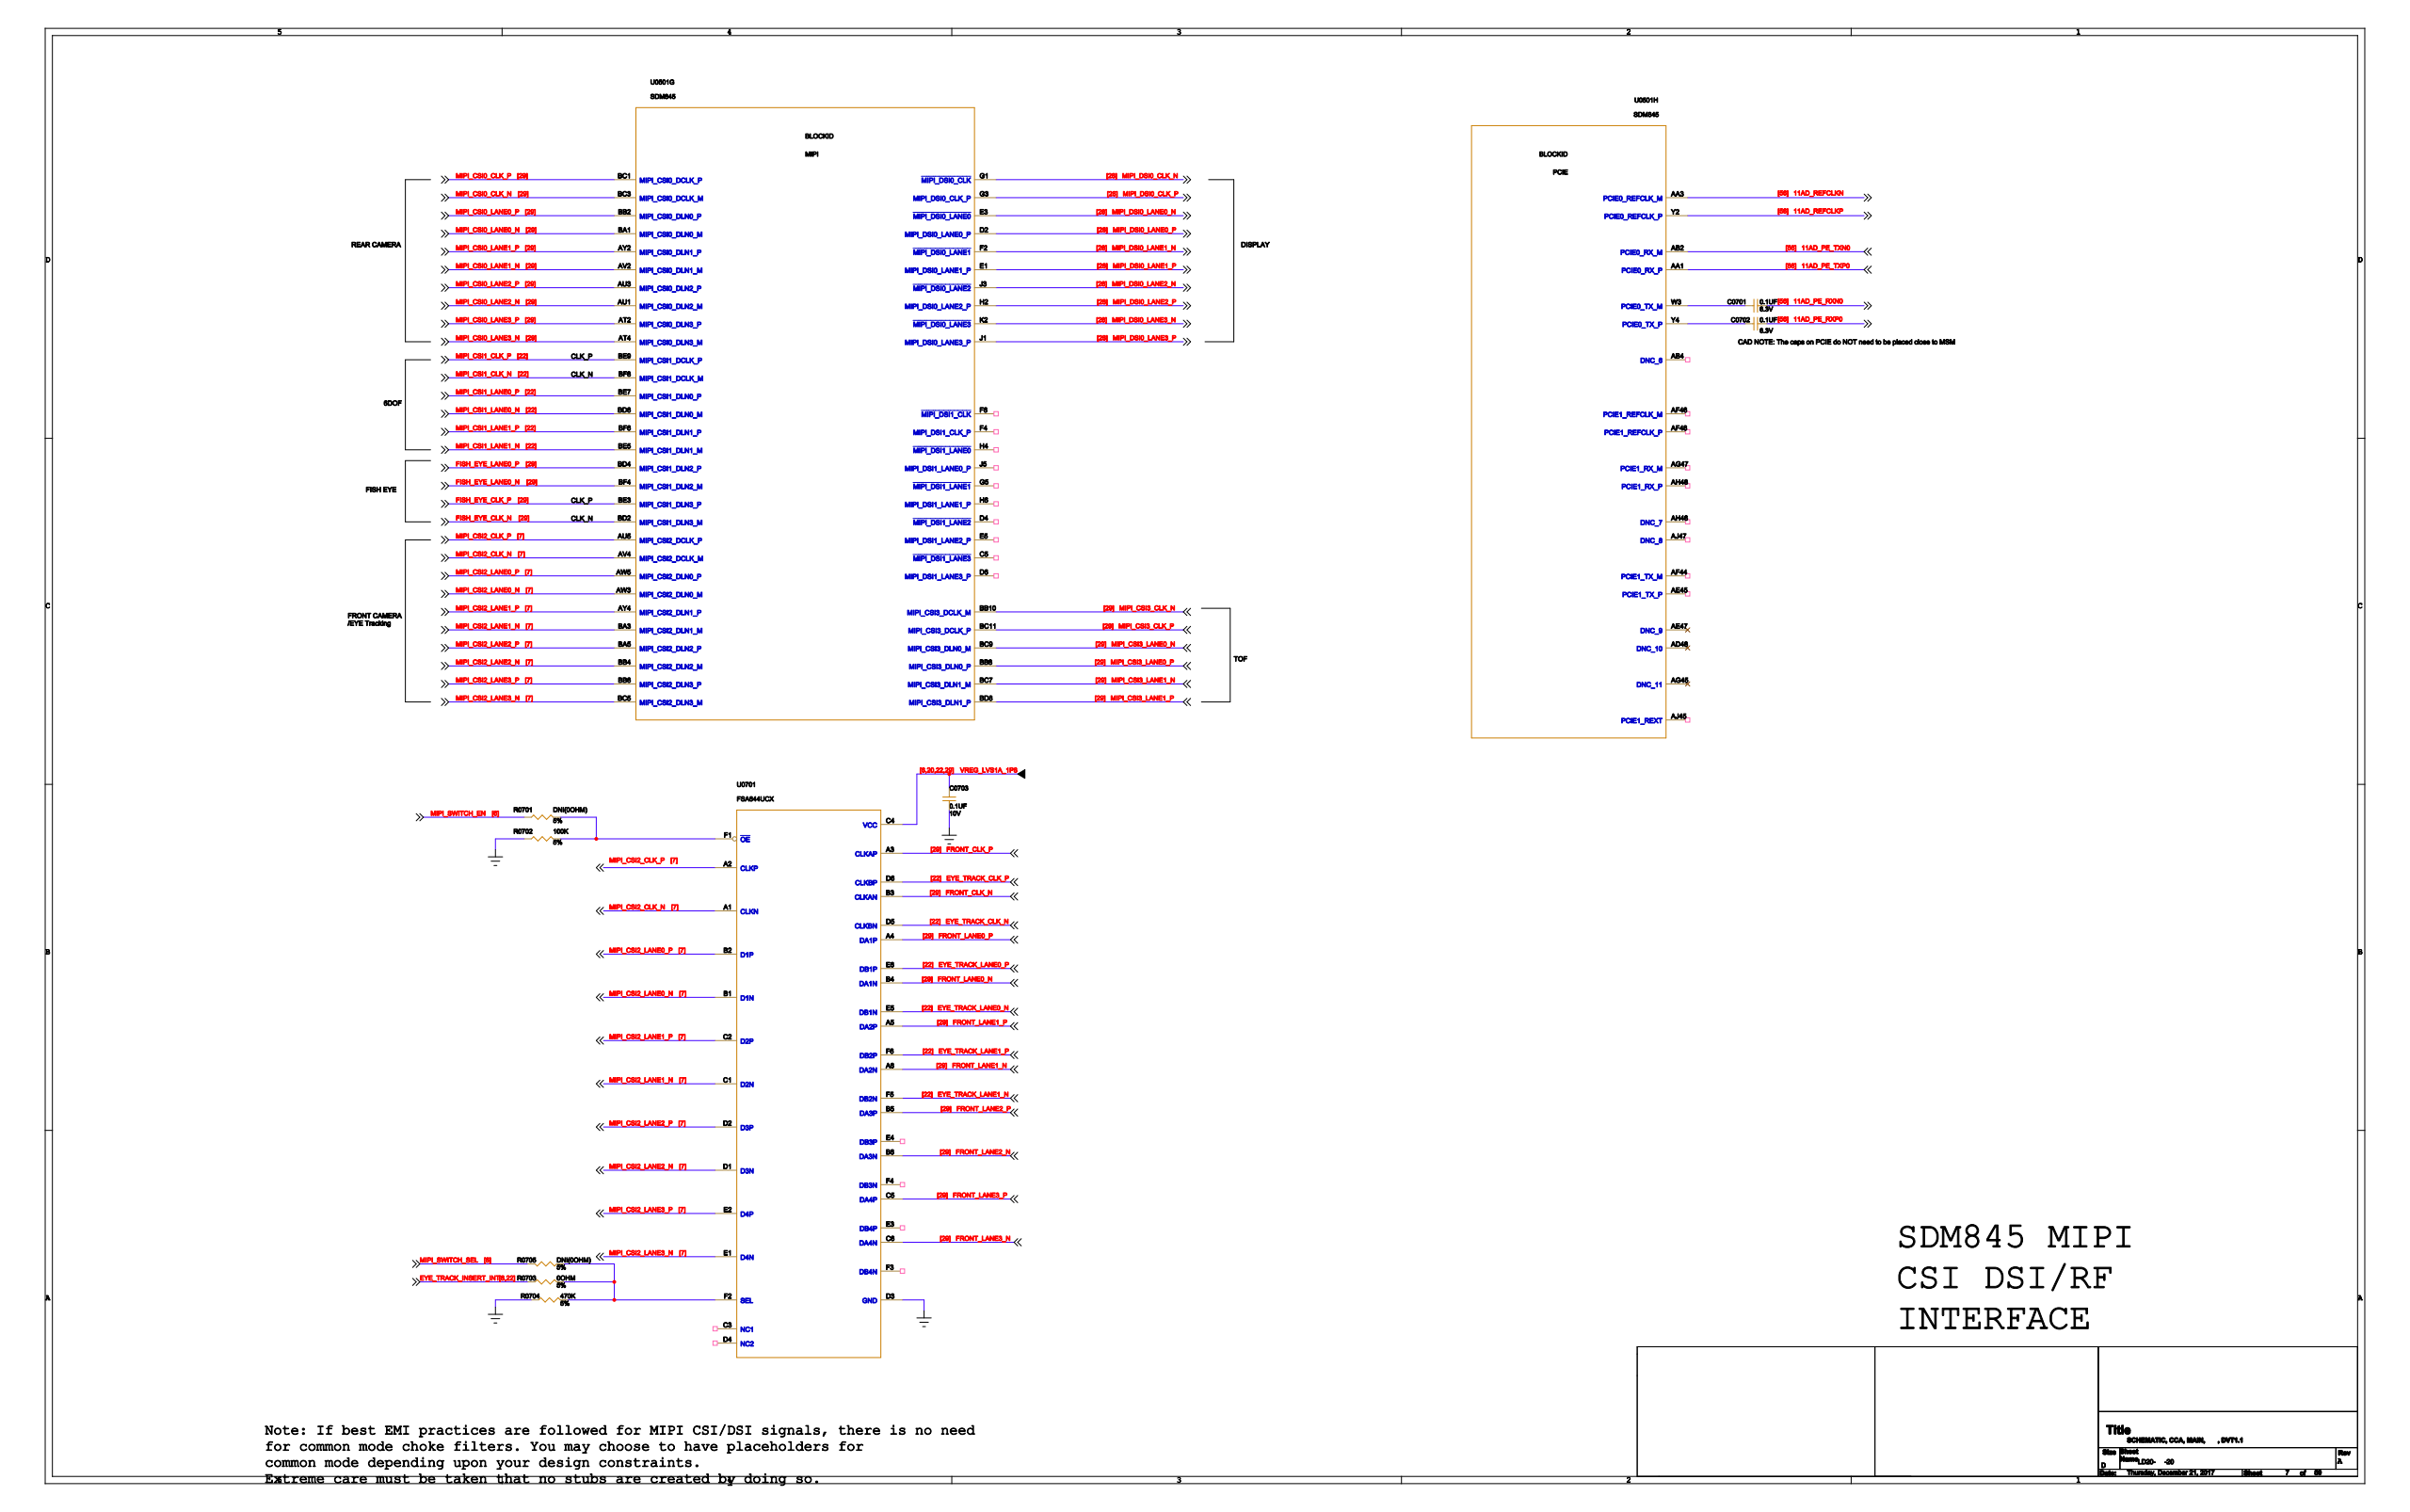Circuit board | Cadence Allegro | 1520 parts | 1149 nets | one sheet of the schematic
Parts on this sheet (reference | value | footprint):
C0701 | 0.1UF | 2P0201R
C0702 | 0.1UF | 2P0201R
C0703 | 0.1UF | 2P0201R
R0701 | DNI(0OHM) | 2P0201R_DNI
R0702 | 100K | 2P0201R
R0703 | 0OHM | 2P0201R
R0704 | 470K | 2P0201R
R0705 | DNI(0OHM) | 2P0201R_DNI
U0501 | SDM845 | 914PGA490X490B138D45
U0701 | FSA644UCX | 36PGA94X94B157
Nets of these parts (net: part-pin ...):
GND: C0703-2 R0702-2 R0704-2 U0501-A1 U0501-A3 U0501-A5 U0501-B2 U0501-B4 U0501-B6 U0501-C1 U0501-C3 U0701-D3
11AD_PE_RXN0: C0701-2
11AD_PE_RXP0: C0702-2
11AD_PE_TXN0: U0501-AB2
11AD_PE_TXP0: U0501-AA1
11AD_REFCLKN: U0501-AA3
11AD_REFCLKP: U0501-Y2
EYE_TRACK_INSERT_INT: R0703-2
EYE_TRACK_LANE0_P: U0701-E6
EYE_TRACK_LANE0_N: U0701-E5
EYE_TRACK_CLK_P: U0701-D6
EYE_TRACK_CLK_N: U0701-D5
EYE_TRACK_LANE1_P: U0701-F6
EYE_TRACK_LANE1_N: U0701-F5
MIPI_CSI1_CLK_P: U0501-BE9
MIPI_CSI1_CLK_N: U0501-BF8
VREG_LVS1A_1P8: C0703-1 U0701-C4
MIPI_CSI1_LANE0_N: U0501-BD6
MIPI_CSI1_LANE0_P: U0501-BE7
MIPI_CSI1_LANE1_P: U0501-BF6
MIPI_CSI1_LANE1_N: U0501-BE5
N48971381: R0703-1 R0704-1 R0705-2 U0701-F2
MIPI_CSI0_LANE2_N: U0501-AU1
MIPI_CSI0_LANE2_P: U0501-AU3
MIPI_CSI0_LANE0_N: U0501-BA1
MIPI_CSI0_LANE0_P: U0501-BB2
MIPI_CSI0_CLK_P: U0501-BC1
MIPI_CSI0_CLK_N: U0501-BC3
MIPI_CSI0_LANE1_N: U0501-AV2
MIPI_CSI0_LANE1_P: U0501-AY2
MIPI_CSI0_LANE3_P: U0501-AT2
MIPI_CSI0_LANE3_N: U0501-AT4
FRONT_CLK_N: U0701-B3
FRONT_CLK_P: U0701-A3
MIPI_CSI2_CLK_N: U0501-AV4 U0701-A1
MIPI_CSI2_CLK_P: U0501-AU5 U0701-A2
MIPI_CSI2_LANE0_N: U0501-AW3 U0701-B1
MIPI_CSI2_LANE0_P: U0501-AW5 U0701-B2
MIPI_CSI2_LANE1_N: U0501-BA3 U0701-C1
MIPI_CSI2_LANE1_P: U0501-AY4 U0701-C2
MIPI_CSI2_LANE2_N: U0501-BB4 U0701-D1
MIPI_CSI2_LANE2_P: U0501-BA5 U0701-D2
MIPI_CSI2_LANE3_N: U0501-BC5 U0701-E1
MIPI_CSI2_LANE3_P: U0501-BB6 U0701-E2
FRONT_LANE0_N: U0701-B4
FRONT_LANE0_P: U0701-A4
FRONT_LANE1_N: U0701-A6
FRONT_LANE1_P: U0701-A5
FRONT_LANE2_N: U0701-B6
FRONT_LANE2_P: U0701-B5
FRONT_LANE3_N: U0701-C6
FRONT_LANE3_P: U0701-C5
N48971157: R0701-1 R0702-1 U0701-F1
N47128251: C0701-1 U0501-W3
N47128254: C0702-1 U0501-Y4
MIPI_DSI0_CLK_P: U0501-G3
MIPI_DSI0_CLK_N: U0501-G1
MIPI_DSI0_LANE0_P: U0501-D2
MIPI_DSI0_LANE0_N: U0501-E3
MIPI_DSI0_LANE1_P: U0501-E1
MIPI_DSI0_LANE1_N: U0501-F2
MIPI_DSI0_LANE2_P: U0501-H2
MIPI_DSI0_LANE2_N: U0501-J3
MIPI_DSI0_LANE3_P: U0501-J1
MIPI_DSI0_LANE3_N: U0501-K2
FISH_EYE_CLK_P: U0501-BE3
FISH_EYE_CLK_N: U0501-BD2
FISH_EYE_LANE0_P: U0501-BD4
FISH_EYE_LANE0_N: U0501-BF4
MIPI_CSI3_LANE0_P: U0501-BB8
MIPI_CSI3_LANE0_N: U0501-BC9
MIPI_CSI3_CLK_P: U0501-BC11
MIPI_CSI3_CLK_N: U0501-BB10
MIPI_CSI3_LANE1_P: U0501-BD8
MIPI_CSI3_LANE1_N: U0501-BC7
MIPI_SWITCH_SEL: R0705-1
MIPI_SWITCH_EN: R0701-2